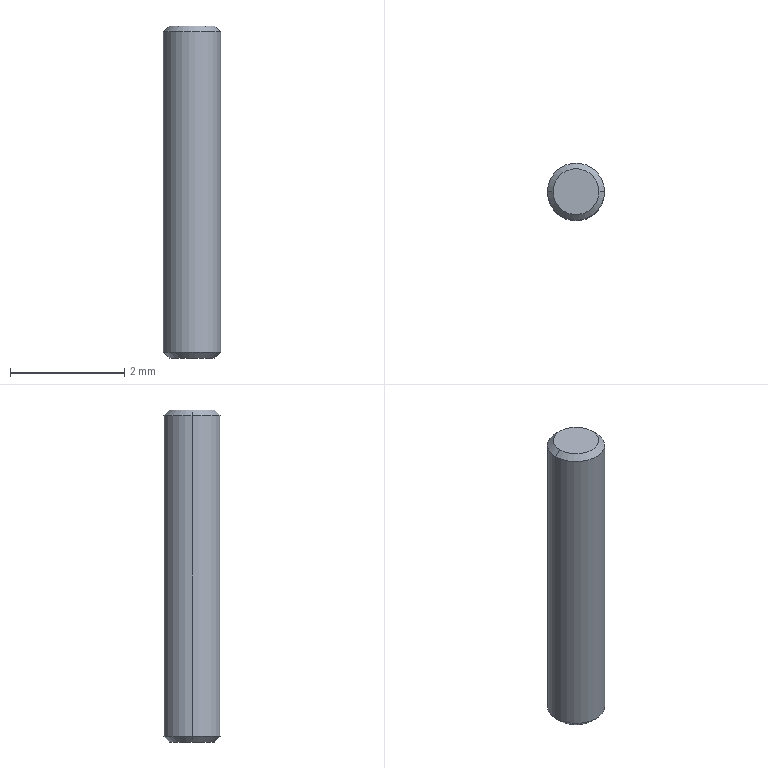Part | SolidWorks | features Chamfer 1, Extrusion 1 | 1 solid | 8 faces | box 1 x 1 x 5.8 mm | volume 4.526 mm3 | cone 4 | cylinder 2 | plane 2 | commonest cylinder face diameters 1 x2
STEP:
#1=CARTESIAN_POINT('',(0.4,0.,2.9));
#2=VERTEX_POINT('',#1);
#3=CARTESIAN_POINT('',(-0.4,0.,2.9));
#4=VERTEX_POINT('',#3);
#5=CARTESIAN_POINT('',(0.,0.,2.9));
#6=DIRECTION('',(0.,0.,1.));
#7=DIRECTION('',(1.,0.,0.));
#8=AXIS2_PLACEMENT_3D('',#5,#6,#7);
#9=CIRCLE('',#8,0.4);
#10=EDGE_CURVE('',#2,#4,#9,.T.);
#11=ORIENTED_EDGE('',*,*,#10,.F.);
#12=CARTESIAN_POINT('',(0.5,0.,2.8));
#13=VERTEX_POINT('',#12);
#14=CARTESIAN_POINT('',(0.4,0.,2.9));
#15=DIRECTION('',(0.7071,0.,-0.7071));
#16=VECTOR('',#15,1000.);
#17=LINE('',#14,#16);
#18=EDGE_CURVE('',#2,#13,#17,.T.);
#19=ORIENTED_EDGE('',*,*,#18,.T.);
#20=CARTESIAN_POINT('',(-0.5,0.,2.8));
#21=VERTEX_POINT('',#20);
#22=CARTESIAN_POINT('',(0.,0.,2.8));
#23=DIRECTION('',(0.,0.,-1.));
#24=DIRECTION('',(1.,0.,0.));
#25=AXIS2_PLACEMENT_3D('',#22,#23,#24);
#26=CIRCLE('',#25,0.5);
#27=EDGE_CURVE('',#21,#13,#26,.T.);
#28=ORIENTED_EDGE('',*,*,#27,.F.);
#29=CARTESIAN_POINT('',(-0.4,0.,2.9));
#30=DIRECTION('',(-0.7071,0.,-0.7071));
#31=VECTOR('',#30,1000.);
#32=LINE('',#29,#31);
#33=EDGE_CURVE('',#4,#21,#32,.T.);
#34=ORIENTED_EDGE('',*,*,#33,.F.);
#35=EDGE_LOOP('',(#11,#19,#28,#34));
#36=FACE_OUTER_BOUND('',#35,.T.);
#37=CARTESIAN_POINT('',(0.,0.,2.9));
#38=DIRECTION('',(0.,0.,-1.));
#39=DIRECTION('',(-1.,0.,0.));
#40=AXIS2_PLACEMENT_3D('',#37,#38,#39);
#41=CONICAL_SURFACE('',#40,0.4,0.7854);
#42=ADVANCED_FACE('',(#36),#41,.T.);
#43=CARTESIAN_POINT('',(-0.4,0.,-2.9));
#44=VERTEX_POINT('',#43);
#45=CARTESIAN_POINT('',(0.4,0.,-2.9));
#46=VERTEX_POINT('',#45);
#47=CARTESIAN_POINT('',(0.,0.,-2.9));
#48=DIRECTION('',(0.,0.,-1.));
#49=DIRECTION('',(1.,0.,0.));
#50=AXIS2_PLACEMENT_3D('',#47,#48,#49);
#51=CIRCLE('',#50,0.4);
#52=EDGE_CURVE('',#44,#46,#51,.T.);
#53=ORIENTED_EDGE('',*,*,#52,.F.);
#54=CARTESIAN_POINT('',(-0.5,0.,-2.8));
#55=VERTEX_POINT('',#54);
#56=CARTESIAN_POINT('',(-0.5,0.,-2.8));
#57=DIRECTION('',(-0.7071,0.,0.7071));
#58=VECTOR('',#57,1000.);
#59=LINE('',#56,#58);
#60=EDGE_CURVE('',#44,#55,#59,.T.);
#61=ORIENTED_EDGE('',*,*,#60,.T.);
#62=CARTESIAN_POINT('',(0.5,0.,-2.8));
#63=VERTEX_POINT('',#62);
#64=CARTESIAN_POINT('',(0.,0.,-2.8));
#65=DIRECTION('',(0.,0.,1.));
#66=DIRECTION('',(1.,0.,0.));
#67=AXIS2_PLACEMENT_3D('',#64,#65,#66);
#68=CIRCLE('',#67,0.5);
#69=EDGE_CURVE('',#63,#55,#68,.T.);
#70=ORIENTED_EDGE('',*,*,#69,.F.);
#71=CARTESIAN_POINT('',(0.5,0.,-2.8));
#72=DIRECTION('',(0.7071,0.,0.7071));
#73=VECTOR('',#72,1000.);
#74=LINE('',#71,#73);
#75=EDGE_CURVE('',#46,#63,#74,.T.);
#76=ORIENTED_EDGE('',*,*,#75,.F.);
#77=EDGE_LOOP('',(#53,#61,#70,#76));
#78=FACE_OUTER_BOUND('',#77,.T.);
#79=CARTESIAN_POINT('',(0.,0.,-2.8));
#80=DIRECTION('',(0.,0.,1.));
#81=DIRECTION('',(1.,0.,0.));
#82=AXIS2_PLACEMENT_3D('',#79,#80,#81);
#83=CONICAL_SURFACE('',#82,0.5,0.7854);
#84=ADVANCED_FACE('',(#78),#83,.T.);
#85=ORIENTED_EDGE('',*,*,#27,.T.);
#86=CARTESIAN_POINT('',(0.5,0.,2.9));
#87=DIRECTION('',(0.,0.,-1.));
#88=VECTOR('',#87,1000.);
#89=LINE('',#86,#88);
#90=EDGE_CURVE('',#13,#63,#89,.T.);
#91=ORIENTED_EDGE('',*,*,#90,.T.);
#92=ORIENTED_EDGE('',*,*,#69,.T.);
#93=CARTESIAN_POINT('',(-0.5,0.,2.9));
#94=DIRECTION('',(0.,0.,-1.));
#95=VECTOR('',#94,1000.);
#96=LINE('',#93,#95);
#97=EDGE_CURVE('',#21,#55,#96,.T.);
#98=ORIENTED_EDGE('',*,*,#97,.F.);
#99=EDGE_LOOP('',(#85,#91,#92,#98));
#100=FACE_OUTER_BOUND('',#99,.T.);
#101=CARTESIAN_POINT('',(0.,0.,2.9));
#102=DIRECTION('',(0.,0.,-1.));
#103=DIRECTION('',(-1.,0.,0.));
#104=AXIS2_PLACEMENT_3D('',#101,#102,#103);
#105=CYLINDRICAL_SURFACE('',#104,0.5);
#106=ADVANCED_FACE('',(#100),#105,.T.);
#107=ORIENTED_EDGE('',*,*,#90,.F.);
#108=CARTESIAN_POINT('',(0.,0.,2.8));
#109=DIRECTION('',(0.,0.,-1.));
#110=DIRECTION('',(1.,0.,0.));
#111=AXIS2_PLACEMENT_3D('',#108,#109,#110);
#112=CIRCLE('',#111,0.5);
#113=EDGE_CURVE('',#13,#21,#112,.T.);
#114=ORIENTED_EDGE('',*,*,#113,.T.);
#115=ORIENTED_EDGE('',*,*,#97,.T.);
#116=CARTESIAN_POINT('',(0.,0.,-2.8));
#117=DIRECTION('',(0.,0.,1.));
#118=DIRECTION('',(1.,0.,0.));
#119=AXIS2_PLACEMENT_3D('',#116,#117,#118);
#120=CIRCLE('',#119,0.5);
#121=EDGE_CURVE('',#55,#63,#120,.T.);
#122=ORIENTED_EDGE('',*,*,#121,.T.);
#123=EDGE_LOOP('',(#107,#114,#115,#122));
#124=FACE_OUTER_BOUND('',#123,.T.);
#125=CARTESIAN_POINT('',(0.,0.,2.9));
#126=DIRECTION('',(0.,0.,-1.));
#127=DIRECTION('',(-1.,0.,0.));
#128=AXIS2_PLACEMENT_3D('',#125,#126,#127);
#129=CYLINDRICAL_SURFACE('',#128,0.5);
#130=ADVANCED_FACE('',(#124),#129,.T.);
#131=CARTESIAN_POINT('',(0.,0.,2.9));
#132=DIRECTION('',(0.,0.,1.));
#133=DIRECTION('',(1.,0.,0.));
#134=AXIS2_PLACEMENT_3D('',#131,#132,#133);
#135=CIRCLE('',#134,0.4);
#136=EDGE_CURVE('',#4,#2,#135,.T.);
#137=ORIENTED_EDGE('',*,*,#136,.T.);
#138=ORIENTED_EDGE('',*,*,#10,.T.);
#139=EDGE_LOOP('',(#137,#138));
#140=FACE_OUTER_BOUND('',#139,.T.);
#141=CARTESIAN_POINT('',(0.,0.,2.9));
#142=DIRECTION('',(0.,0.,1.));
#143=DIRECTION('',(1.,0.,0.));
#144=AXIS2_PLACEMENT_3D('',#141,#142,#143);
#145=PLANE('',#144);
#146=ADVANCED_FACE('',(#140),#145,.T.);
#147=CARTESIAN_POINT('',(0.,0.,-2.9));
#148=DIRECTION('',(0.,0.,-1.));
#149=DIRECTION('',(1.,0.,0.));
#150=AXIS2_PLACEMENT_3D('',#147,#148,#149);
#151=CIRCLE('',#150,0.4);
#152=EDGE_CURVE('',#46,#44,#151,.T.);
#153=ORIENTED_EDGE('',*,*,#152,.T.);
#154=ORIENTED_EDGE('',*,*,#52,.T.);
#155=EDGE_LOOP('',(#153,#154));
#156=FACE_OUTER_BOUND('',#155,.T.);
#157=CARTESIAN_POINT('',(0.,0.,-2.9));
#158=DIRECTION('',(0.,0.,1.));
#159=DIRECTION('',(1.,0.,0.));
#160=AXIS2_PLACEMENT_3D('',#157,#158,#159);
#161=PLANE('',#160);
#162=ADVANCED_FACE('',(#156),#161,.F.);
#163=ORIENTED_EDGE('',*,*,#60,.F.);
#164=ORIENTED_EDGE('',*,*,#152,.F.);
#165=ORIENTED_EDGE('',*,*,#75,.T.);
#166=ORIENTED_EDGE('',*,*,#121,.F.);
#167=EDGE_LOOP('',(#163,#164,#165,#166));
#168=FACE_OUTER_BOUND('',#167,.T.);
#169=CARTESIAN_POINT('',(0.,0.,-2.8));
#170=DIRECTION('',(0.,0.,1.));
#171=DIRECTION('',(1.,0.,0.));
#172=AXIS2_PLACEMENT_3D('',#169,#170,#171);
#173=CONICAL_SURFACE('',#172,0.5,0.7854);
#174=ADVANCED_FACE('',(#168),#173,.T.);
#175=ORIENTED_EDGE('',*,*,#18,.F.);
#176=ORIENTED_EDGE('',*,*,#136,.F.);
#177=ORIENTED_EDGE('',*,*,#33,.T.);
#178=ORIENTED_EDGE('',*,*,#113,.F.);
#179=EDGE_LOOP('',(#175,#176,#177,#178));
#180=FACE_OUTER_BOUND('',#179,.T.);
#181=CARTESIAN_POINT('',(0.,0.,2.9));
#182=DIRECTION('',(0.,0.,-1.));
#183=DIRECTION('',(-1.,0.,0.));
#184=AXIS2_PLACEMENT_3D('',#181,#182,#183);
#185=CONICAL_SURFACE('',#184,0.4,0.7854);
#186=ADVANCED_FACE('',(#180),#185,.T.);
#187=CLOSED_SHELL('',(#42,#84,#106,#130,#146,#162,#174,#186));
#188=MANIFOLD_SOLID_BREP('',#187);
#189=CARTESIAN_POINT('',(0.,0.,0.));
#190=DIRECTION('',(0.,0.,1.));
#191=DIRECTION('',(1.,0.,0.));
#192=AXIS2_PLACEMENT_3D('',#189,#190,#191);
#193=(LENGTH_UNIT()NAMED_UNIT(*)SI_UNIT(.MILLI.,.METRE.));
#194=UNCERTAINTY_MEASURE_WITH_UNIT(LENGTH_MEASURE(0.00001),#193,'','');
#195=(NAMED_UNIT(*)PLANE_ANGLE_UNIT()SI_UNIT($,.RADIAN.));
#196=(NAMED_UNIT(*)SI_UNIT($,.STERADIAN.)SOLID_ANGLE_UNIT());
#197=(GEOMETRIC_REPRESENTATION_CONTEXT(3)GLOBAL_UNCERTAINTY_ASSIGNED_CONTEXT((#194))GLOBAL_UNIT_ASSIGNED_CONTEXT((#193,#195,#196))REPRESENTATION_CONTEXT('',''));
#198=ADVANCED_BREP_SHAPE_REPRESENTATION('',(#188,#192),#197);